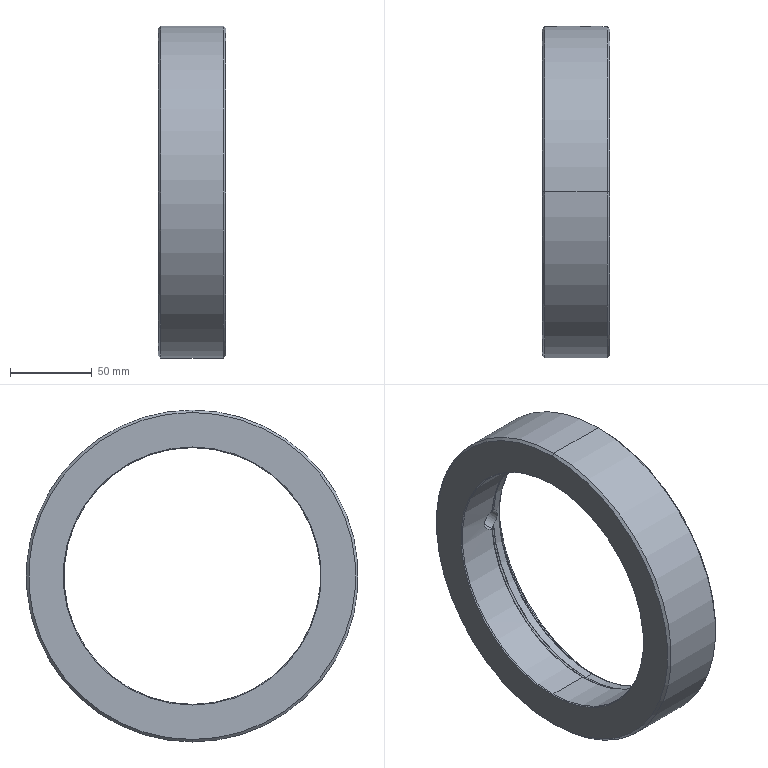Part | SolidWorks | features Chamfer 2, 3DProfileFeature 1, HoleWzd 1, Revolution 1 | 1 solid | 36 faces | box 41.402 x 203.2 x 203.2 mm | volume 502742 mm3 | torus 12 | cone 11 | cylinder 10 | plane 3 | commonest cylinder face diameters 12.573 x2 157.099 x2 160.274 x2 172.974 x2 203.2 x2
STEP:
#1=CARTESIAN_POINT('',(26.314,78.319,-6.287));
#2=VERTEX_POINT('',#1);
#3=CARTESIAN_POINT('',(26.136,78.298,-6.284));
#4=VERTEX_POINT('',#3);
#5=CARTESIAN_POINT('',(26.314,78.319,-6.287));
#6=CARTESIAN_POINT('',(26.256,78.305,-6.287));
#7=CARTESIAN_POINT('',(26.196,78.298,-6.286));
#8=CARTESIAN_POINT('',(26.136,78.298,-6.284));
#9=B_SPLINE_CURVE_WITH_KNOTS('',3,(#5,#6,#7,#8),.UNSPECIFIED.,.F.,.F.,(4,4),(0.0002182,0.0003967),.UNSPECIFIED.);
#10=EDGE_CURVE('',#2,#4,#9,.T.);
#11=ORIENTED_EDGE('',*,*,#10,.F.);
#12=CARTESIAN_POINT('',(26.314,101.405,-6.287));
#13=VERTEX_POINT('',#12);
#14=CARTESIAN_POINT('',(26.314,101.6,-6.287));
#15=DIRECTION('',(0.,1.,0.));
#16=VECTOR('',#15,1000.);
#17=LINE('',#14,#16);
#18=EDGE_CURVE('',#2,#13,#17,.T.);
#19=ORIENTED_EDGE('',*,*,#18,.T.);
#20=CARTESIAN_POINT('',(26.314,101.405,6.287));
#21=VERTEX_POINT('',#20);
#22=CARTESIAN_POINT('',(26.314,101.405,6.287));
#23=CARTESIAN_POINT('',(25.899,101.405,6.287));
#24=CARTESIAN_POINT('',(25.49,101.408,6.246));
#25=CARTESIAN_POINT('',(24.888,101.415,6.126));
#26=CARTESIAN_POINT('',(24.688,101.418,6.076));
#27=CARTESIAN_POINT('',(24.293,101.425,5.956));
#28=CARTESIAN_POINT('',(24.097,101.429,5.886));
#29=CARTESIAN_POINT('',(23.526,101.443,5.649));
#30=CARTESIAN_POINT('',(23.165,101.454,5.456));
#31=CARTESIAN_POINT('',(22.482,101.477,5.));
#32=CARTESIAN_POINT('',(22.158,101.49,4.734));
#33=CARTESIAN_POINT('',(21.578,101.515,4.154));
#34=CARTESIAN_POINT('',(21.318,101.528,3.838));
#35=CARTESIAN_POINT('',(20.974,101.546,3.323));
#36=CARTESIAN_POINT('',(20.867,101.552,3.144));
#37=CARTESIAN_POINT('',(20.673,101.562,2.781));
#38=CARTESIAN_POINT('',(20.497,101.572,2.41));
#39=CARTESIAN_POINT('',(20.359,101.58,2.025));
#40=CARTESIAN_POINT('',(20.24,101.587,1.631));
#41=CARTESIAN_POINT('',(20.189,101.59,1.429));
#42=CARTESIAN_POINT('',(20.068,101.597,0.8204));
#43=CARTESIAN_POINT('',(20.028,101.6,0.4124));
#44=CARTESIAN_POINT('',(20.028,101.6,-0.4079));
#45=CARTESIAN_POINT('',(20.069,101.597,-0.8245));
#46=CARTESIAN_POINT('',(20.229,101.588,-1.631));
#47=CARTESIAN_POINT('',(20.348,101.581,-2.023));
#48=CARTESIAN_POINT('',(20.584,101.567,-2.594));
#49=CARTESIAN_POINT('',(20.673,101.562,-2.782));
#50=CARTESIAN_POINT('',(20.868,101.551,-3.146));
#51=CARTESIAN_POINT('',(20.974,101.546,-3.322));
#52=CARTESIAN_POINT('',(21.315,101.528,-3.833));
#53=CARTESIAN_POINT('',(21.575,101.516,-4.151));
#54=CARTESIAN_POINT('',(22.162,101.49,-4.738));
#55=CARTESIAN_POINT('',(22.48,101.477,-4.998));
#56=CARTESIAN_POINT('',(22.99,101.46,-5.34));
#57=CARTESIAN_POINT('',(23.166,101.454,-5.445));
#58=CARTESIAN_POINT('',(23.53,101.443,-5.64));
#59=CARTESIAN_POINT('',(23.718,101.438,-5.729));
#60=CARTESIAN_POINT('',(24.29,101.425,-5.966));
#61=CARTESIAN_POINT('',(24.682,101.418,-6.085));
#62=CARTESIAN_POINT('',(25.487,101.408,-6.245));
#63=CARTESIAN_POINT('',(25.904,101.405,-6.287));
#64=CARTESIAN_POINT('',(26.314,101.405,-6.287));
#65=B_SPLINE_CURVE_WITH_KNOTS('',3,(#22,#23,#24,#25,#26,#27,#28,#29,#30,#31,#32,#33,#34,#35,#36,#37,#38,#39,#40,#41,#42,#43,#44,#45,#46,#47,#48,#49,#50,#51,#52,#53,#54,#55,#56,#57,#58,#59,#60,#61,#62,#63,#64),.UNSPECIFIED.,.F.,.F.,(4,2,2,2,2,2,2,2,1,2,2,2,2,2,2,2,2,2,2,2,2,4),(0.,0.001229,0.001843,0.002457,0.003686,0.004915,0.006144,0.006758,0.007372,0.007987,0.008601,0.00983,0.01106,0.01229,0.0129,0.01352,0.01474,0.01597,0.01659,0.0172,0.01843,0.01966),.UNSPECIFIED.);
#66=EDGE_CURVE('',#21,#13,#65,.T.);
#67=ORIENTED_EDGE('',*,*,#66,.F.);
#68=CARTESIAN_POINT('',(26.314,78.319,6.287));
#69=VERTEX_POINT('',#68);
#70=CARTESIAN_POINT('',(26.314,101.6,6.287));
#71=DIRECTION('',(0.,1.,0.));
#72=VECTOR('',#71,1000.);
#73=LINE('',#70,#72);
#74=EDGE_CURVE('',#69,#21,#73,.T.);
#75=ORIENTED_EDGE('',*,*,#74,.F.);
#76=CARTESIAN_POINT('',(26.136,78.298,6.284));
#77=VERTEX_POINT('',#76);
#78=CARTESIAN_POINT('',(26.136,78.298,6.284));
#79=CARTESIAN_POINT('',(26.196,78.298,6.286));
#80=CARTESIAN_POINT('',(26.256,78.305,6.287));
#81=CARTESIAN_POINT('',(26.314,78.319,6.287));
#82=B_SPLINE_CURVE_WITH_KNOTS('',3,(#78,#79,#80,#81),.UNSPECIFIED.,.F.,.F.,(4,4),(0.000000197,0.00018),.UNSPECIFIED.);
#83=EDGE_CURVE('',#77,#69,#82,.T.);
#84=ORIENTED_EDGE('',*,*,#83,.F.);
#85=CARTESIAN_POINT('',(26.136,78.298,-6.284));
#86=CARTESIAN_POINT('',(25.728,78.299,-6.272));
#87=CARTESIAN_POINT('',(25.328,78.303,-6.222));
#88=CARTESIAN_POINT('',(24.739,78.313,-6.089));
#89=CARTESIAN_POINT('',(24.545,78.317,-6.036));
#90=CARTESIAN_POINT('',(24.16,78.327,-5.909));
#91=CARTESIAN_POINT('',(23.969,78.332,-5.836));
#92=CARTESIAN_POINT('',(23.413,78.35,-5.592));
#93=CARTESIAN_POINT('',(23.062,78.364,-5.395));
#94=CARTESIAN_POINT('',(22.4,78.395,-4.936));
#95=CARTESIAN_POINT('',(22.086,78.411,-4.67));
#96=CARTESIAN_POINT('',(21.525,78.443,-4.092));
#97=CARTESIAN_POINT('',(21.274,78.459,-3.778));
#98=CARTESIAN_POINT('',(20.941,78.482,-3.27));
#99=CARTESIAN_POINT('',(20.838,78.489,-3.093));
#100=CARTESIAN_POINT('',(20.65,78.502,-2.735));
#101=CARTESIAN_POINT('',(20.565,78.508,-2.552));
#102=CARTESIAN_POINT('',(20.338,78.525,-1.993));
#103=CARTESIAN_POINT('',(20.223,78.534,-1.607));
#104=CARTESIAN_POINT('',(20.066,78.546,-0.8059));
#105=CARTESIAN_POINT('',(20.028,78.549,-0.4046));
#106=CARTESIAN_POINT('',(20.028,78.55,0.1989));
#107=CARTESIAN_POINT('',(20.037,78.549,0.4003));
#108=CARTESIAN_POINT('',(20.076,78.546,0.8036));
#109=CARTESIAN_POINT('',(20.106,78.543,1.006));
#110=CARTESIAN_POINT('',(20.222,78.534,1.603));
#111=CARTESIAN_POINT('',(20.337,78.525,1.988));
#112=CARTESIAN_POINT('',(20.64,78.503,2.735));
#113=CARTESIAN_POINT('',(20.83,78.489,3.099));
#114=CARTESIAN_POINT('',(21.271,78.46,3.774));
#115=CARTESIAN_POINT('',(21.522,78.444,4.088));
#116=CARTESIAN_POINT('',(21.945,78.419,4.524));
#117=CARTESIAN_POINT('',(22.094,78.411,4.664));
#118=CARTESIAN_POINT('',(22.403,78.395,4.926));
#119=CARTESIAN_POINT('',(22.563,78.387,5.048));
#120=CARTESIAN_POINT('',(23.058,78.365,5.392));
#121=CARTESIAN_POINT('',(23.41,78.351,5.59));
#122=CARTESIAN_POINT('',(24.156,78.326,5.918));
#123=CARTESIAN_POINT('',(24.539,78.317,6.044));
#124=CARTESIAN_POINT('',(25.323,78.303,6.221));
#125=CARTESIAN_POINT('',(25.728,78.299,6.272));
#126=CARTESIAN_POINT('',(26.136,78.298,6.284));
#127=B_SPLINE_CURVE_WITH_KNOTS('',3,(#85,#86,#87,#88,#89,#90,#91,#92,#93,#94,#95,#96,#97,#98,#99,#100,#101,#102,#103,#104,#105,#106,#107,#108,#109,#110,#111,#112,#113,#114,#115,#116,#117,#118,#119,#120,#121,#122,#123,#124,#125,#126),.UNSPECIFIED.,.F.,.F.,(4,2,2,2,2,2,2,2,2,2,2,2,2,2,2,2,2,2,2,2,4),(0.,0.001207,0.00181,0.002413,0.00362,0.004826,0.006033,0.006636,0.007239,0.008446,0.009653,0.01026,0.01086,0.01207,0.01327,0.01448,0.01508,0.01569,0.01689,0.0181,0.01931),.UNSPECIFIED.);
#128=EDGE_CURVE('',#4,#77,#127,.T.);
#129=ORIENTED_EDGE('',*,*,#128,.F.);
#130=EDGE_LOOP('',(#11,#19,#67,#75,#84,#129));
#131=FACE_OUTER_BOUND('',#130,.T.);
#132=CARTESIAN_POINT('',(26.314,101.6,0.));
#133=DIRECTION('',(0.,1.,0.));
#134=DIRECTION('',(0.,0.,1.));
#135=AXIS2_PLACEMENT_3D('',#132,#133,#134);
#136=CYLINDRICAL_SURFACE('',#135,6.287);
#137=ADVANCED_FACE('',(#131),#136,.F.);
#138=CARTESIAN_POINT('',(0.,0.,100.076));
#139=VERTEX_POINT('',#138);
#140=CARTESIAN_POINT('',(0.,0.,-100.076));
#141=VERTEX_POINT('',#140);
#142=CARTESIAN_POINT('',(0.,0.,0.));
#143=DIRECTION('',(-1.,0.,0.));
#144=DIRECTION('',(0.,0.,-1.));
#145=AXIS2_PLACEMENT_3D('',#142,#143,#144);
#146=CIRCLE('',#145,100.076);
#147=EDGE_CURVE('',#139,#141,#146,.T.);
#148=ORIENTED_EDGE('',*,*,#147,.F.);
#149=CARTESIAN_POINT('',(1.524,0.,101.6));
#150=VERTEX_POINT('',#149);
#151=CARTESIAN_POINT('',(0.,0.,100.076));
#152=DIRECTION('',(0.7071,0.,0.7071));
#153=VECTOR('',#152,1000.);
#154=LINE('',#151,#153);
#155=EDGE_CURVE('',#139,#150,#154,.T.);
#156=ORIENTED_EDGE('',*,*,#155,.T.);
#157=CARTESIAN_POINT('',(1.524,0.,-101.6));
#158=VERTEX_POINT('',#157);
#159=CARTESIAN_POINT('',(1.524,0.,0.));
#160=DIRECTION('',(1.,0.,0.));
#161=DIRECTION('',(0.,0.,-1.));
#162=AXIS2_PLACEMENT_3D('',#159,#160,#161);
#163=CIRCLE('',#162,101.6);
#164=EDGE_CURVE('',#158,#150,#163,.T.);
#165=ORIENTED_EDGE('',*,*,#164,.F.);
#166=CARTESIAN_POINT('',(0.,0.,-100.076));
#167=DIRECTION('',(0.7071,0.,-0.7071));
#168=VECTOR('',#167,1000.);
#169=LINE('',#166,#168);
#170=EDGE_CURVE('',#141,#158,#169,.T.);
#171=ORIENTED_EDGE('',*,*,#170,.F.);
#172=EDGE_LOOP('',(#148,#156,#165,#171));
#173=FACE_OUTER_BOUND('',#172,.T.);
#174=CARTESIAN_POINT('',(0.,0.,0.));
#175=DIRECTION('',(1.,0.,0.));
#176=DIRECTION('',(0.,0.,-1.));
#177=AXIS2_PLACEMENT_3D('',#174,#175,#176);
#178=CONICAL_SURFACE('',#177,100.076,0.7854);
#179=ADVANCED_FACE('',(#173),#178,.T.);
#180=CARTESIAN_POINT('',(41.402,0.,-100.076));
#181=VERTEX_POINT('',#180);
#182=CARTESIAN_POINT('',(41.402,0.,100.076));
#183=VERTEX_POINT('',#182);
#184=CARTESIAN_POINT('',(41.402,0.,0.));
#185=DIRECTION('',(1.,0.,0.));
#186=DIRECTION('',(0.,0.,1.));
#187=AXIS2_PLACEMENT_3D('',#184,#185,#186);
#188=CIRCLE('',#187,100.076);
#189=EDGE_CURVE('',#181,#183,#188,.T.);
#190=ORIENTED_EDGE('',*,*,#189,.F.);
#191=CARTESIAN_POINT('',(39.878,0.,-101.6));
#192=VERTEX_POINT('',#191);
#193=CARTESIAN_POINT('',(39.878,0.,-101.6));
#194=DIRECTION('',(-0.7071,0.,-0.7071));
#195=VECTOR('',#194,1000.);
#196=LINE('',#193,#195);
#197=EDGE_CURVE('',#181,#192,#196,.T.);
#198=ORIENTED_EDGE('',*,*,#197,.T.);
#199=CARTESIAN_POINT('',(39.878,0.,101.6));
#200=VERTEX_POINT('',#199);
#201=CARTESIAN_POINT('',(39.878,0.,0.));
#202=DIRECTION('',(-1.,0.,0.));
#203=DIRECTION('',(0.,0.,1.));
#204=AXIS2_PLACEMENT_3D('',#201,#202,#203);
#205=CIRCLE('',#204,101.6);
#206=EDGE_CURVE('',#200,#192,#205,.T.);
#207=ORIENTED_EDGE('',*,*,#206,.F.);
#208=CARTESIAN_POINT('',(39.878,0.,101.6));
#209=DIRECTION('',(-0.7071,0.,0.7071));
#210=VECTOR('',#209,1000.);
#211=LINE('',#208,#210);
#212=EDGE_CURVE('',#183,#200,#211,.T.);
#213=ORIENTED_EDGE('',*,*,#212,.F.);
#214=EDGE_LOOP('',(#190,#198,#207,#213));
#215=FACE_OUTER_BOUND('',#214,.T.);
#216=CARTESIAN_POINT('',(39.878,0.,0.));
#217=DIRECTION('',(-1.,0.,0.));
#218=DIRECTION('',(0.,0.,1.));
#219=AXIS2_PLACEMENT_3D('',#216,#217,#218);
#220=CONICAL_SURFACE('',#219,101.6,0.7854);
#221=ADVANCED_FACE('',(#215),#220,.T.);
#222=CARTESIAN_POINT('',(0.762,0.,-78.549));
#223=VERTEX_POINT('',#222);
#224=CARTESIAN_POINT('',(0.762,0.,78.549));
#225=VERTEX_POINT('',#224);
#226=CARTESIAN_POINT('',(0.762,0.,0.));
#227=DIRECTION('',(-1.,0.,0.));
#228=DIRECTION('',(0.,0.,-1.));
#229=AXIS2_PLACEMENT_3D('',#226,#227,#228);
#230=CIRCLE('',#229,78.549);
#231=EDGE_CURVE('',#223,#225,#230,.T.);
#232=ORIENTED_EDGE('',*,*,#231,.F.);
#233=CARTESIAN_POINT('',(0.,0.,-78.989));
#234=VERTEX_POINT('',#233);
#235=CARTESIAN_POINT('',(0.762,0.,-78.549));
#236=DIRECTION('',(-0.866,0.,-0.5));
#237=VECTOR('',#236,1000.);
#238=LINE('',#235,#237);
#239=EDGE_CURVE('',#223,#234,#238,.T.);
#240=ORIENTED_EDGE('',*,*,#239,.T.);
#241=CARTESIAN_POINT('',(0.,0.,78.989));
#242=VERTEX_POINT('',#241);
#243=CARTESIAN_POINT('',(0.,0.,0.));
#244=DIRECTION('',(1.,0.,0.));
#245=DIRECTION('',(0.,0.,-1.));
#246=AXIS2_PLACEMENT_3D('',#243,#244,#245);
#247=CIRCLE('',#246,78.989);
#248=EDGE_CURVE('',#242,#234,#247,.T.);
#249=ORIENTED_EDGE('',*,*,#248,.F.);
#250=CARTESIAN_POINT('',(0.762,0.,78.549));
#251=DIRECTION('',(-0.866,0.,0.5));
#252=VECTOR('',#251,1000.);
#253=LINE('',#250,#252);
#254=EDGE_CURVE('',#225,#242,#253,.T.);
#255=ORIENTED_EDGE('',*,*,#254,.F.);
#256=EDGE_LOOP('',(#232,#240,#249,#255));
#257=FACE_OUTER_BOUND('',#256,.T.);
#258=CARTESIAN_POINT('',(0.762,0.,0.));
#259=DIRECTION('',(-1.,0.,0.));
#260=DIRECTION('',(0.,0.,1.));
#261=AXIS2_PLACEMENT_3D('',#258,#259,#260);
#262=CONICAL_SURFACE('',#261,78.549,0.5236);
#263=ADVANCED_FACE('',(#257),#262,.F.);
#264=CARTESIAN_POINT('',(26.136,0.,-78.549));
#265=VERTEX_POINT('',#264);
#266=CARTESIAN_POINT('',(26.136,0.,78.549));
#267=VERTEX_POINT('',#266);
#268=CARTESIAN_POINT('',(26.136,0.,0.));
#269=DIRECTION('',(-1.,0.,0.));
#270=DIRECTION('',(0.,0.,1.));
#271=AXIS2_PLACEMENT_3D('',#268,#269,#270);
#272=CIRCLE('',#271,78.549);
#273=EDGE_CURVE('',#265,#267,#272,.T.);
#274=ORIENTED_EDGE('',*,*,#273,.F.);
#275=CARTESIAN_POINT('',(-48.08,0.,-78.549));
#276=DIRECTION('',(-1.,0.,0.));
#277=VECTOR('',#276,1000.);
#278=LINE('',#275,#277);
#279=EDGE_CURVE('',#265,#223,#278,.T.);
#280=ORIENTED_EDGE('',*,*,#279,.T.);
#281=ORIENTED_EDGE('',*,*,#231,.T.);
#282=CARTESIAN_POINT('',(-48.08,0.,78.549));
#283=DIRECTION('',(-1.,0.,0.));
#284=VECTOR('',#283,1000.);
#285=LINE('',#282,#284);
#286=EDGE_CURVE('',#267,#225,#285,.T.);
#287=ORIENTED_EDGE('',*,*,#286,.F.);
#288=EDGE_LOOP('',(#274,#280,#281,#287));
#289=FACE_OUTER_BOUND('',#288,.T.);
#290=CARTESIAN_POINT('',(-48.08,0.,0.));
#291=DIRECTION('',(-1.,0.,0.));
#292=DIRECTION('',(0.,0.,1.));
#293=AXIS2_PLACEMENT_3D('',#290,#291,#292);
#294=CYLINDRICAL_SURFACE('',#293,78.549);
#295=ADVANCED_FACE('',(#289),#294,.F.);
#296=CARTESIAN_POINT('',(26.136,0.,0.));
#297=DIRECTION('',(-1.,0.,0.));
#298=DIRECTION('',(0.,0.,1.));
#299=AXIS2_PLACEMENT_3D('',#296,#297,#298);
#300=CIRCLE('',#299,78.549);
#301=EDGE_CURVE('',#4,#265,#300,.T.);
#302=ORIENTED_EDGE('',*,*,#301,.T.);
#303=CARTESIAN_POINT('',(26.517,0.,-78.652));
#304=VERTEX_POINT('',#303);
#305=CARTESIAN_POINT('',(26.136,0.,-79.311));
#306=DIRECTION('',(0.,1.,0.));
#307=DIRECTION('',(0.,0.,1.));
#308=AXIS2_PLACEMENT_3D('',#305,#306,#307);
#309=CIRCLE('',#308,0.762);
#310=EDGE_CURVE('',#265,#304,#309,.T.);
#311=ORIENTED_EDGE('',*,*,#310,.T.);
#312=CARTESIAN_POINT('',(26.517,78.4,-6.283));
#313=VERTEX_POINT('',#312);
#314=CARTESIAN_POINT('',(26.517,0.,0.));
#315=DIRECTION('',(-1.,0.,0.));
#316=DIRECTION('',(0.,0.,1.));
#317=AXIS2_PLACEMENT_3D('',#314,#315,#316);
#318=CIRCLE('',#317,78.652);
#319=EDGE_CURVE('',#313,#304,#318,.T.);
#320=ORIENTED_EDGE('',*,*,#319,.F.);
#321=CARTESIAN_POINT('',(26.517,78.4,-6.283));
#322=CARTESIAN_POINT('',(26.453,78.363,-6.285));
#323=CARTESIAN_POINT('',(26.386,78.336,-6.287));
#324=CARTESIAN_POINT('',(26.314,78.319,-6.287));
#325=B_SPLINE_CURVE_WITH_KNOTS('',3,(#321,#322,#323,#324),.UNSPECIFIED.,.F.,.F.,(4,4),(0.000000228,0.0002182),.UNSPECIFIED.);
#326=EDGE_CURVE('',#313,#2,#325,.T.);
#327=ORIENTED_EDGE('',*,*,#326,.T.);
#328=ORIENTED_EDGE('',*,*,#10,.T.);
#329=EDGE_LOOP('',(#302,#311,#320,#327,#328));
#330=FACE_OUTER_BOUND('',#329,.T.);
#331=CARTESIAN_POINT('',(26.136,0.,0.));
#332=DIRECTION('',(-1.,0.,0.));
#333=DIRECTION('',(0.,0.,1.));
#334=AXIS2_PLACEMENT_3D('',#331,#332,#333);
#335=TOROIDAL_SURFACE('',#334,79.311,0.762);
#336=ADVANCED_FACE('',(#330),#335,.T.);
#337=ORIENTED_EDGE('',*,*,#310,.F.);
#338=ORIENTED_EDGE('',*,*,#273,.T.);
#339=CARTESIAN_POINT('',(26.517,0.,78.652));
#340=VERTEX_POINT('',#339);
#341=CARTESIAN_POINT('',(26.136,0.,79.311));
#342=DIRECTION('',(0.,-1.,0.));
#343=DIRECTION('',(0.,0.,-1.));
#344=AXIS2_PLACEMENT_3D('',#341,#342,#343);
#345=CIRCLE('',#344,0.762);
#346=EDGE_CURVE('',#267,#340,#345,.T.);
#347=ORIENTED_EDGE('',*,*,#346,.T.);
#348=CARTESIAN_POINT('',(26.517,0.,0.));
#349=DIRECTION('',(-1.,0.,0.));
#350=DIRECTION('',(0.,0.,1.));
#351=AXIS2_PLACEMENT_3D('',#348,#349,#350);
#352=CIRCLE('',#351,78.652);
#353=EDGE_CURVE('',#304,#340,#352,.T.);
#354=ORIENTED_EDGE('',*,*,#353,.F.);
#355=EDGE_LOOP('',(#337,#338,#347,#354));
#356=FACE_OUTER_BOUND('',#355,.T.);
#357=CARTESIAN_POINT('',(26.136,0.,0.));
#358=DIRECTION('',(-1.,0.,0.));
#359=DIRECTION('',(0.,0.,1.));
#360=AXIS2_PLACEMENT_3D('',#357,#358,#359);
#361=TOROIDAL_SURFACE('',#360,79.311,0.762);
#362=ADVANCED_FACE('',(#356),#361,.T.);
#363=ORIENTED_EDGE('',*,*,#353,.T.);
#364=CARTESIAN_POINT('',(28.913,0.,80.035));
#365=VERTEX_POINT('',#364);
#366=CARTESIAN_POINT('',(26.517,0.,78.652));
#367=DIRECTION('',(0.866,0.,0.5));
#368=VECTOR('',#367,1000.);
#369=LINE('',#366,#368);
#370=EDGE_CURVE('',#340,#365,#369,.T.);
#371=ORIENTED_EDGE('',*,*,#370,.T.);
#372=CARTESIAN_POINT('',(28.913,0.,-80.035));
#373=VERTEX_POINT('',#372);
#374=CARTESIAN_POINT('',(28.913,0.,0.));
#375=DIRECTION('',(-1.,0.,0.));
#376=DIRECTION('',(0.,0.,1.));
#377=AXIS2_PLACEMENT_3D('',#374,#375,#376);
#378=CIRCLE('',#377,80.035);
#379=EDGE_CURVE('',#373,#365,#378,.T.);
#380=ORIENTED_EDGE('',*,*,#379,.F.);
#381=CARTESIAN_POINT('',(26.517,0.,-78.652));
#382=DIRECTION('',(0.866,0.,-0.5));
#383=VECTOR('',#382,1000.);
#384=LINE('',#381,#383);
#385=EDGE_CURVE('',#304,#373,#384,.T.);
#386=ORIENTED_EDGE('',*,*,#385,.F.);
#387=EDGE_LOOP('',(#363,#371,#380,#386));
#388=FACE_OUTER_BOUND('',#387,.T.);
#389=CARTESIAN_POINT('',(26.517,0.,0.));
#390=DIRECTION('',(1.,0.,0.));
#391=DIRECTION('',(0.,0.,-1.));
#392=AXIS2_PLACEMENT_3D('',#389,#390,#391);
#393=CONICAL_SURFACE('',#392,78.652,0.5236);
#394=ADVANCED_FACE('',(#388),#393,.F.);
#395=ORIENTED_EDGE('',*,*,#319,.T.);
#396=ORIENTED_EDGE('',*,*,#385,.T.);
#397=CARTESIAN_POINT('',(28.913,79.83,-5.725));
#398=VERTEX_POINT('',#397);
#399=CARTESIAN_POINT('',(28.913,0.,0.));
#400=DIRECTION('',(-1.,0.,0.));
#401=DIRECTION('',(0.,0.,1.));
#402=AXIS2_PLACEMENT_3D('',#399,#400,#401);
#403=CIRCLE('',#402,80.035);
#404=EDGE_CURVE('',#398,#373,#403,.T.);
#405=ORIENTED_EDGE('',*,*,#404,.F.);
#406=CARTESIAN_POINT('',(28.913,79.83,-5.725));
#407=CARTESIAN_POINT('',(28.532,79.597,-5.897));
#408=CARTESIAN_POINT('',(28.142,79.361,-6.029));
#409=CARTESIAN_POINT('',(27.343,78.884,-6.215));
#410=CARTESIAN_POINT('',(26.932,78.642,-6.27));
#411=CARTESIAN_POINT('',(26.517,78.4,-6.283));
#412=B_SPLINE_CURVE_WITH_KNOTS('',3,(#406,#407,#408,#409,#410,#411),.UNSPECIFIED.,.F.,.F.,(4,2,4),(0.0003004,0.001723,0.003145),.UNSPECIFIED.);
#413=EDGE_CURVE('',#398,#313,#412,.T.);
#414=ORIENTED_EDGE('',*,*,#413,.T.);
#415=EDGE_LOOP('',(#395,#396,#405,#414));
#416=FACE_OUTER_BOUND('',#415,.T.);
#417=CARTESIAN_POINT('',(26.517,0.,0.));
#418=DIRECTION('',(1.,0.,0.));
#419=DIRECTION('',(0.,0.,-1.));
#420=AXIS2_PLACEMENT_3D('',#417,#418,#419);
#421=CONICAL_SURFACE('',#420,78.652,0.5236);
#422=ADVANCED_FACE('',(#416),#421,.F.);
#423=CARTESIAN_POINT('',(29.294,0.,-80.137));
#424=VERTEX_POINT('',#423);
#425=CARTESIAN_POINT('',(29.294,0.,80.137));
#426=VERTEX_POINT('',#425);
#427=CARTESIAN_POINT('',(29.294,0.,0.));
#428=DIRECTION('',(-1.,0.,0.));
#429=DIRECTION('',(0.,0.,1.));
#430=AXIS2_PLACEMENT_3D('',#427,#428,#429);
#431=CIRCLE('',#430,80.137);
#432=EDGE_CURVE('',#424,#426,#431,.T.);
#433=ORIENTED_EDGE('',*,*,#432,.F.);
#434=CARTESIAN_POINT('',(29.294,0.,-79.375));
#435=DIRECTION('',(0.,1.,0.));
#436=DIRECTION('',(0.,0.,1.));
#437=AXIS2_PLACEMENT_3D('',#434,#435,#436);
#438=CIRCLE('',#437,0.762);
#439=EDGE_CURVE('',#424,#373,#438,.T.);
#440=ORIENTED_EDGE('',*,*,#439,.T.);
#441=ORIENTED_EDGE('',*,*,#379,.T.);
#442=CARTESIAN_POINT('',(29.294,0.,79.375));
#443=DIRECTION('',(0.,-1.,0.));
#444=DIRECTION('',(0.,0.,-1.));
#445=AXIS2_PLACEMENT_3D('',#442,#443,#444);
#446=CIRCLE('',#445,0.762);
#447=EDGE_CURVE('',#426,#365,#446,.T.);
#448=ORIENTED_EDGE('',*,*,#447,.F.);
#449=EDGE_LOOP('',(#433,#440,#441,#448));
#450=FACE_OUTER_BOUND('',#449,.T.);
#451=CARTESIAN_POINT('',(29.294,0.,0.));
#452=DIRECTION('',(-1.,0.,0.));
#453=DIRECTION('',(0.,0.,1.));
#454=AXIS2_PLACEMENT_3D('',#451,#452,#453);
#455=TOROIDAL_SURFACE('',#454,79.375,0.762);
#456=ADVANCED_FACE('',(#450),#455,.F.);
#457=CARTESIAN_POINT('',(29.294,79.946,5.536));
#458=VERTEX_POINT('',#457);
#459=CARTESIAN_POINT('',(29.294,0.,0.));
#460=DIRECTION('',(-1.,0.,0.));
#461=DIRECTION('',(0.,0.,1.));
#462=AXIS2_PLACEMENT_3D('',#459,#460,#461);
#463=CIRCLE('',#462,80.137);
#464=EDGE_CURVE('',#426,#458,#463,.T.);
#465=ORIENTED_EDGE('',*,*,#464,.F.);
#466=ORIENTED_EDGE('',*,*,#447,.T.);
#467=CARTESIAN_POINT('',(28.913,79.83,5.725));
#468=VERTEX_POINT('',#467);
#469=CARTESIAN_POINT('',(28.913,0.,0.));
#470=DIRECTION('',(-1.,0.,0.));
#471=DIRECTION('',(0.,0.,1.));
#472=AXIS2_PLACEMENT_3D('',#469,#470,#471);
#473=CIRCLE('',#472,80.035);
#474=EDGE_CURVE('',#365,#468,#473,.T.);
#475=ORIENTED_EDGE('',*,*,#474,.T.);
#476=CARTESIAN_POINT('',(28.913,79.83,5.725));
#477=CARTESIAN_POINT('',(29.032,79.903,5.671));
#478=CARTESIAN_POINT('',(29.162,79.941,5.607));
#479=CARTESIAN_POINT('',(29.294,79.946,5.536));
#480=B_SPLINE_CURVE_WITH_KNOTS('',3,(#476,#477,#478,#479),.UNSPECIFIED.,.F.,.F.,(4,4),(0.000000248,0.0004419),.UNSPECIFIED.);
#481=EDGE_CURVE('',#468,#458,#480,.T.);
#482=ORIENTED_EDGE('',*,*,#481,.T.);
#483=EDGE_LOOP('',(#465,#466,#475,#482));
#484=FACE_OUTER_BOUND('',#483,.T.);
#485=CARTESIAN_POINT('',(29.294,0.,0.));
#486=DIRECTION('',(-1.,0.,0.));
#487=DIRECTION('',(0.,0.,1.));
#488=AXIS2_PLACEMENT_3D('',#485,#486,#487);
#489=TOROIDAL_SURFACE('',#488,79.375,0.762);
#490=ADVANCED_FACE('',(#484),#489,.F.);
#491=CARTESIAN_POINT('',(34.163,0.,-80.137));
#492=VERTEX_POINT('',#491);
#493=CARTESIAN_POINT('',(34.163,0.,80.137));
#494=VERTEX_POINT('',#493);
#495=CARTESIAN_POINT('',(34.163,0.,0.));
#496=DIRECTION('',(-1.,0.,0.));
#497=DIRECTION('',(0.,0.,1.));
#498=AXIS2_PLACEMENT_3D('',#495,#496,#497);
#499=CIRCLE('',#498,80.137);
#500=EDGE_CURVE('',#492,#494,#499,.T.);
#501=ORIENTED_EDGE('',*,*,#500,.F.);
#502=CARTESIAN_POINT('',(-48.08,0.,-80.137));
#503=DIRECTION('',(-1.,0.,0.));
#504=VECTOR('',#503,1000.);
#505=LINE('',#502,#504);
#506=EDGE_CURVE('',#492,#424,#505,.T.);
#507=ORIENTED_EDGE('',*,*,#506,.T.);
#508=ORIENTED_EDGE('',*,*,#432,.T.);
#509=CARTESIAN_POINT('',(-48.08,0.,80.137));
#510=DIRECTION('',(-1.,0.,0.));
#511=VECTOR('',#510,1000.);
#512=LINE('',#509,#511);
#513=EDGE_CURVE('',#494,#426,#512,.T.);
#514=ORIENTED_EDGE('',*,*,#513,.F.);
#515=EDGE_LOOP('',(#501,#507,#508,#514));
#516=FACE_OUTER_BOUND('',#515,.T.);
#517=CARTESIAN_POINT('',(-48.08,0.,0.));
#518=DIRECTION('',(-1.,0.,0.));
#519=DIRECTION('',(0.,0.,1.));
#520=AXIS2_PLACEMENT_3D('',#517,#518,#519);
#521=CYLINDRICAL_SURFACE('',#520,80.137);
#522=ADVANCED_FACE('',(#516),#521,.F.);
#523=CARTESIAN_POINT('',(34.163,0.,0.));
#524=DIRECTION('',(-1.,0.,0.));
#525=DIRECTION('',(0.,0.,1.));
#526=AXIS2_PLACEMENT_3D('',#523,#524,#525);
#527=CIRCLE('',#526,80.137);
#528=EDGE_CURVE('',#494,#492,#527,.T.);
#529=ORIENTED_EDGE('',*,*,#528,.T.);
#530=CARTESIAN_POINT('',(34.925,0.,-80.899));
#531=VERTEX_POINT('',#530);
#532=CARTESIAN_POINT('',(34.163,0.,-80.899));
#533=DIRECTION('',(0.,1.,0.));
#534=DIRECTION('',(0.,0.,1.));
#535=AXIS2_PLACEMENT_3D('',#532,#533,#534);
#536=CIRCLE('',#535,0.762);
#537=EDGE_CURVE('',#492,#531,#536,.T.);
#538=ORIENTED_EDGE('',*,*,#537,.T.);
#539=CARTESIAN_POINT('',(34.925,0.,80.899));
#540=VERTEX_POINT('',#539);
#541=CARTESIAN_POINT('',(34.925,0.,0.));
#542=DIRECTION('',(-1.,0.,0.));
#543=DIRECTION('',(0.,0.,1.));
#544=AXIS2_PLACEMENT_3D('',#541,#542,#543);
#545=CIRCLE('',#544,80.899);
#546=EDGE_CURVE('',#540,#531,#545,.T.);
#547=ORIENTED_EDGE('',*,*,#546,.F.);
#548=CARTESIAN_POINT('',(34.163,0.,80.899));
#549=DIRECTION('',(0.,-1.,0.));
#550=DIRECTION('',(0.,0.,-1.));
#551=AXIS2_PLACEMENT_3D('',#548,#549,#550);
#552=CIRCLE('',#551,0.762);
#553=EDGE_CURVE('',#494,#540,#552,.T.);
#554=ORIENTED_EDGE('',*,*,#553,.F.);
#555=EDGE_LOOP('',(#529,#538,#547,#554));
#556=FACE_OUTER_BOUND('',#555,.T.);
#557=CARTESIAN_POINT('',(34.163,0.,0.));
#558=DIRECTION('',(-1.,0.,0.));
#559=DIRECTION('',(0.,0.,1.));
#560=AXIS2_PLACEMENT_3D('',#557,#558,#559);
#561=TOROIDAL_SURFACE('',#560,80.899,0.762);
#562=ADVANCED_FACE('',(#556),#561,.T.);
#563=CARTESIAN_POINT('',(35.884,0.,-86.893));
#564=VERTEX_POINT('',#563);
#565=CARTESIAN_POINT('',(35.884,0.,86.893));
#566=VERTEX_POINT('',#565);
#567=CARTESIAN_POINT('',(35.884,0.,0.));
#568=DIRECTION('',(-1.,0.,0.));
#569=DIRECTION('',(0.,0.,1.));
#570=AXIS2_PLACEMENT_3D('',#567,#568,#569);
#571=CIRCLE('',#570,86.893);
#572=EDGE_CURVE('',#564,#566,#571,.T.);
#573=ORIENTED_EDGE('',*,*,#572,.F.);
#574=CARTESIAN_POINT('',(34.925,0.,-86.157));
#575=VERTEX_POINT('',#574);
#576=CARTESIAN_POINT('',(35.687,0.,-86.157));
#577=DIRECTION('',(0.,1.,0.));
#578=DIRECTION('',(0.,0.,1.));
#579=AXIS2_PLACEMENT_3D('',#576,#577,#578);
#580=CIRCLE('',#579,0.762);
#581=EDGE_CURVE('',#564,#575,#580,.T.);
#582=ORIENTED_EDGE('',*,*,#581,.T.);
#583=CARTESIAN_POINT('',(34.925,0.,86.157));
#584=VERTEX_POINT('',#583);
#585=CARTESIAN_POINT('',(34.925,0.,0.));
#586=DIRECTION('',(-1.,0.,0.));
#587=DIRECTION('',(0.,0.,1.));
#588=AXIS2_PLACEMENT_3D('',#585,#586,#587);
#589=CIRCLE('',#588,86.157);
#590=EDGE_CURVE('',#575,#584,#589,.T.);
#591=ORIENTED_EDGE('',*,*,#590,.T.);
#592=CARTESIAN_POINT('',(35.687,0.,86.157));
#593=DIRECTION('',(0.,-1.,0.));
#594=DIRECTION('',(0.,0.,-1.));
#595=AXIS2_PLACEMENT_3D('',#592,#593,#594);
#596=CIRCLE('',#595,0.762);
#597=EDGE_CURVE('',#566,#584,#596,.T.);
#598=ORIENTED_EDGE('',*,*,#597,.F.);
#599=EDGE_LOOP('',(#573,#582,#591,#598));
#600=FACE_OUTER_BOUND('',#599,.T.);
#601=CARTESIAN_POINT('',(35.687,0.,0.));
#602=DIRECTION('',(-1.,0.,0.));
#603=DIRECTION('',(0.,0.,1.));
#604=AXIS2_PLACEMENT_3D('',#601,#602,#603);
#605=TOROIDAL_SURFACE('',#604,86.157,0.762);
#606=ADVANCED_FACE('',(#600),#605,.F.);
#607=CARTESIAN_POINT('',(37.401,0.,-86.487));
#608=VERTEX_POINT('',#607);
#609=CARTESIAN_POINT('',(37.401,0.,86.487));
#610=VERTEX_POINT('',#609);
#611=CARTESIAN_POINT('',(37.401,0.,0.));
#612=DIRECTION('',(-1.,0.,0.));
#613=DIRECTION('',(0.,0.,1.));
#614=AXIS2_PLACEMENT_3D('',#611,#612,#613);
#615=CIRCLE('',#614,86.487);
#616=EDGE_CURVE('',#608,#610,#615,.T.);
#617=ORIENTED_EDGE('',*,*,#616,.F.);
#618=CARTESIAN_POINT('',(35.884,0.,-86.893));
#619=DIRECTION('',(-0.9659,0.,-0.2588));
#620=VECTOR('',#619,1000.);
#621=LINE('',#618,#620);
#622=EDGE_CURVE('',#608,#564,#621,.T.);
#623=ORIENTED_EDGE('',*,*,#622,.T.);
#624=ORIENTED_EDGE('',*,*,#572,.T.);
#625=CARTESIAN_POINT('',(35.884,0.,86.893));
#626=DIRECTION('',(-0.9659,0.,0.2588));
#627=VECTOR('',#626,1000.);
#628=LINE('',#625,#627);
#629=EDGE_CURVE('',#610,#566,#628,.T.);
#630=ORIENTED_EDGE('',*,*,#629,.F.);
#631=EDGE_LOOP('',(#617,#623,#624,#630));
#632=FACE_OUTER_BOUND('',#631,.T.);
#633=CARTESIAN_POINT('',(35.884,0.,0.));
#634=DIRECTION('',(-1.,0.,0.));
#635=DIRECTION('',(0.,0.,1.));
#636=AXIS2_PLACEMENT_3D('',#633,#634,#635);
#637=CONICAL_SURFACE('',#636,86.893,0.2618);
#638=ADVANCED_FACE('',(#632),#637,.F.);
#639=CARTESIAN_POINT('',(39.878,0.,-86.487));
#640=VERTEX_POINT('',#639);
#641=CARTESIAN_POINT('',(39.878,0.,86.487));
#642=VERTEX_POINT('',#641);
#643=CARTESIAN_POINT('',(39.878,0.,0.));
#644=DIRECTION('',(-1.,0.,0.));
#645=DIRECTION('',(0.,0.,1.));
#646=AXIS2_PLACEMENT_3D('',#643,#644,#645);
#647=CIRCLE('',#646,86.487);
#648=EDGE_CURVE('',#640,#642,#647,.T.);
#649=ORIENTED_EDGE('',*,*,#648,.F.);
#650=CARTESIAN_POINT('',(-48.08,0.,-86.487));
#651=DIRECTION('',(-1.,0.,0.));
#652=VECTOR('',#651,1000.);
#653=LINE('',#650,#652);
#654=EDGE_CURVE('',#640,#608,#653,.T.);
#655=ORIENTED_EDGE('',*,*,#654,.T.);
#656=ORIENTED_EDGE('',*,*,#616,.T.);
#657=CARTESIAN_POINT('',(-48.08,0.,86.487));
#658=DIRECTION('',(-1.,0.,0.));
#659=VECTOR('',#658,1000.);
#660=LINE('',#657,#659);
#661=EDGE_CURVE('',#642,#610,#660,.T.);
#662=ORIENTED_EDGE('',*,*,#661,.F.);
#663=EDGE_LOOP('',(#649,#655,#656,#662));
#664=FACE_OUTER_BOUND('',#663,.T.);
#665=CARTESIAN_POINT('',(-48.08,0.,0.));
#666=DIRECTION('',(-1.,0.,0.));
#667=DIRECTION('',(0.,0.,1.));
#668=AXIS2_PLACEMENT_3D('',#665,#666,#667);
#669=CYLINDRICAL_SURFACE('',#668,86.487);
#670=ADVANCED_FACE('',(#664),#669,.F.);
#671=CARTESIAN_POINT('',(39.878,0.,0.));
#672=DIRECTION('',(-1.,0.,0.));
#673=DIRECTION('',(0.,0.,1.));
#674=AXIS2_PLACEMENT_3D('',#671,#672,#673);
#675=CIRCLE('',#674,86.487);
#676=EDGE_CURVE('',#642,#640,#675,.T.);
#677=ORIENTED_EDGE('',*,*,#676,.T.);
#678=CARTESIAN_POINT('',(41.402,0.,-88.011));
#679=VERTEX_POINT('',#678);
#680=CARTESIAN_POINT('',(39.878,0.,-88.011));
#681=DIRECTION('',(0.,1.,0.));
#682=DIRECTION('',(0.,0.,1.));
#683=AXIS2_PLACEMENT_3D('',#680,#681,#682);
#684=CIRCLE('',#683,1.524);
#685=EDGE_CURVE('',#640,#679,#684,.T.);
#686=ORIENTED_EDGE('',*,*,#685,.T.);
#687=CARTESIAN_POINT('',(41.402,0.,88.011));
#688=VERTEX_POINT('',#687);
#689=CARTESIAN_POINT('',(41.402,0.,0.));
#690=DIRECTION('',(-1.,0.,0.));
#691=DIRECTION('',(0.,0.,1.));
#692=AXIS2_PLACEMENT_3D('',#689,#690,#691);
#693=CIRCLE('',#692,88.011);
#694=EDGE_CURVE('',#688,#679,#693,.T.);
#695=ORIENTED_EDGE('',*,*,#694,.F.);
#696=CARTESIAN_POINT('',(39.878,0.,88.011));
#697=DIRECTION('',(0.,-1.,0.));
#698=DIRECTION('',(0.,0.,-1.));
#699=AXIS2_PLACEMENT_3D('',#696,#697,#698);
#700=CIRCLE('',#699,1.524);
#701=EDGE_CURVE('',#642,#688,#700,.T.);
#702=ORIENTED_EDGE('',*,*,#701,.F.);
#703=EDGE_LOOP('',(#677,#686,#695,#702));
#704=FACE_OUTER_BOUND('',#703,.T.);
#705=CARTESIAN_POINT('',(39.878,0.,0.));
#706=DIRECTION('',(-1.,0.,0.));
#707=DIRECTION('',(0.,0.,1.));
#708=AXIS2_PLACEMENT_3D('',#705,#706,#707);
#709=TOROIDAL_SURFACE('',#708,88.011,1.524);
#710=ADVANCED_FACE('',(#704),#709,.T.);
#711=ORIENTED_EDGE('',*,*,#66,.T.);
#712=CARTESIAN_POINT('',(26.314,101.405,-6.287));
#713=CARTESIAN_POINT('',(26.725,101.405,-6.287));
#714=CARTESIAN_POINT('',(27.132,101.408,-6.247));
#715=CARTESIAN_POINT('',(27.74,101.415,-6.126));
#716=CARTESIAN_POINT('',(27.942,101.418,-6.076));
#717=CARTESIAN_POINT('',(28.336,101.425,-5.956));
#718=CARTESIAN_POINT('',(28.529,101.429,-5.887));
#719=CARTESIAN_POINT('',(29.097,101.443,-5.652));
#720=CARTESIAN_POINT('',(29.462,101.454,-5.458));
#721=CARTESIAN_POINT('',(30.15,101.477,-4.998));
#722=CARTESIAN_POINT('',(30.467,101.49,-4.738));
#723=CARTESIAN_POINT('',(31.047,101.515,-4.159));
#724=CARTESIAN_POINT('',(31.312,101.528,-3.836));
#725=CARTESIAN_POINT('',(31.769,101.552,-3.152));
#726=CARTESIAN_POINT('',(31.962,101.562,-2.792));
#727=CARTESIAN_POINT('',(32.199,101.576,-2.221));
#728=CARTESIAN_POINT('',(32.269,101.58,-2.025));
#729=CARTESIAN_POINT('',(32.389,101.587,-1.63));
#730=CARTESIAN_POINT('',(32.439,101.59,-1.431));
#731=CARTESIAN_POINT('',(32.56,101.597,-0.8281));
#732=CARTESIAN_POINT('',(32.601,101.6,-0.4199));
#733=CARTESIAN_POINT('',(32.601,101.6,0.4097));
#734=CARTESIAN_POINT('',(32.561,101.597,0.8195));
#735=CARTESIAN_POINT('',(32.441,101.59,1.422));
#736=CARTESIAN_POINT('',(32.392,101.587,1.621));
#737=CARTESIAN_POINT('',(32.273,101.58,2.016));
#738=CARTESIAN_POINT('',(32.202,101.576,2.212));
#739=CARTESIAN_POINT('',(31.966,101.563,2.784));
#740=CARTESIAN_POINT('',(31.773,101.552,3.145));
#741=CARTESIAN_POINT('',(31.318,101.528,3.828));
#742=CARTESIAN_POINT('',(31.053,101.516,4.152));
#743=CARTESIAN_POINT('',(30.473,101.49,4.732));
#744=CARTESIAN_POINT('',(30.157,101.478,4.993));
#745=CARTESIAN_POINT('',(29.642,101.46,5.337));
#746=CARTESIAN_POINT('',(29.464,101.454,5.445));
#747=CARTESIAN_POINT('',(29.101,101.443,5.639));
#748=CARTESIAN_POINT('',(28.916,101.439,5.727));
#749=CARTESIAN_POINT('',(28.349,101.425,5.962));
#750=CARTESIAN_POINT('',(27.954,101.418,6.083));
#751=CARTESIAN_POINT('',(27.141,101.408,6.246));
#752=CARTESIAN_POINT('',(26.73,101.405,6.287));
#753=CARTESIAN_POINT('',(26.314,101.405,6.287));
#754=B_SPLINE_CURVE_WITH_KNOTS('',3,(#712,#713,#714,#715,#716,#717,#718,#719,#720,#721,#722,#723,#724,#725,#726,#727,#728,#729,#730,#731,#732,#733,#734,#735,#736,#737,#738,#739,#740,#741,#742,#743,#744,#745,#746,#747,#748,#749,#750,#751,#752,#753),.UNSPECIFIED.,.F.,.F.,(4,2,2,2,2,2,2,2,2,2,2,2,2,2,2,2,2,2,2,2,4),(0.01966,0.02089,0.0215,0.02212,0.02334,0.02457,0.0258,0.02703,0.02764,0.02826,0.02949,0.03072,0.03133,0.03194,0.03317,0.0344,0.03563,0.03624,0.03686,0.03809,0.03931),.UNSPECIFIED.);
#755=EDGE_CURVE('',#13,#21,#754,.T.);
#756=ORIENTED_EDGE('',*,*,#755,.T.);
#757=EDGE_LOOP('',(#711,#756));
#758=FACE_BOUND('',#757,.T.);
#759=ORIENTED_EDGE('',*,*,#206,.T.);
#760=CARTESIAN_POINT('',(-48.08,0.,-101.6));
#761=DIRECTION('',(-1.,0.,0.));
#762=VECTOR('',#761,1000.);
#763=LINE('',#760,#762);
#764=EDGE_CURVE('',#192,#158,#763,.T.);
#765=ORIENTED_EDGE('',*,*,#764,.T.);
#766=ORIENTED_EDGE('',*,*,#164,.T.);
#767=CARTESIAN_POINT('',(-48.08,0.,101.6));
#768=DIRECTION('',(-1.,0.,0.));
#769=VECTOR('',#768,1000.);
#770=LINE('',#767,#769);
#771=EDGE_CURVE('',#200,#150,#770,.T.);
#772=ORIENTED_EDGE('',*,*,#771,.F.);
#773=EDGE_LOOP('',(#759,#765,#766,#772));
#774=FACE_OUTER_BOUND('',#773,.T.);
#775=CARTESIAN_POINT('',(-48.08,0.,0.));
#776=DIRECTION('',(-1.,0.,0.));
#777=DIRECTION('',(0.,0.,1.));
#778=AXIS2_PLACEMENT_3D('',#775,#776,#777);
#779=CYLINDRICAL_SURFACE('',#778,101.6);
#780=ADVANCED_FACE('',(#758,#774),#779,.T.);
#781=CARTESIAN_POINT('',(0.,0.,0.));
#782=DIRECTION('',(-1.,0.,0.));
#783=DIRECTION('',(0.,0.,-1.));
#784=AXIS2_PLACEMENT_3D('',#781,#782,#783);
#785=CIRCLE('',#784,100.076);
#786=EDGE_CURVE('',#141,#139,#785,.T.);
#787=ORIENTED_EDGE('',*,*,#786,.T.);
#788=ORIENTED_EDGE('',*,*,#147,.T.);
#789=EDGE_LOOP('',(#787,#788));
#790=FACE_OUTER_BOUND('',#789,.T.);
#791=ORIENTED_EDGE('',*,*,#248,.T.);
#792=CARTESIAN_POINT('',(0.,0.,0.));
#793=DIRECTION('',(1.,0.,0.));
#794=DIRECTION('',(0.,0.,-1.));
#795=AXIS2_PLACEMENT_3D('',#792,#793,#794);
#796=CIRCLE('',#795,78.989);
#797=EDGE_CURVE('',#234,#242,#796,.T.);
#798=ORIENTED_EDGE('',*,*,#797,.T.);
#799=EDGE_LOOP('',(#791,#798));
#800=FACE_BOUND('',#799,.T.);
#801=CARTESIAN_POINT('',(0.,78.549,0.));
#802=DIRECTION('',(1.,0.,0.));
#803=DIRECTION('',(0.,0.,-1.));
#804=AXIS2_PLACEMENT_3D('',#801,#802,#803);
#805=PLANE('',#804);
#806=ADVANCED_FACE('',(#790,#800),#805,.F.);
#807=ORIENTED_EDGE('',*,*,#764,.F.);
#808=CARTESIAN_POINT('',(39.878,0.,0.));
#809=DIRECTION('',(-1.,0.,0.));
#810=DIRECTION('',(0.,0.,1.));
#811=AXIS2_PLACEMENT_3D('',#808,#809,#810);
#812=CIRCLE('',#811,101.6);
#813=EDGE_CURVE('',#192,#200,#812,.T.);
#814=ORIENTED_EDGE('',*,*,#813,.T.);
#815=ORIENTED_EDGE('',*,*,#771,.T.);
#816=CARTESIAN_POINT('',(1.524,0.,0.));
#817=DIRECTION('',(1.,0.,0.));
#818=DIRECTION('',(0.,0.,-1.));
#819=AXIS2_PLACEMENT_3D('',#816,#817,#818);
#820=CIRCLE('',#819,101.6);
#821=EDGE_CURVE('',#150,#158,#820,.T.);
#822=ORIENTED_EDGE('',*,*,#821,.T.);
#823=EDGE_LOOP('',(#807,#814,#815,#822));
#824=FACE_OUTER_BOUND('',#823,.T.);
#825=CARTESIAN_POINT('',(-48.08,0.,0.));
#826=DIRECTION('',(-1.,0.,0.));
#827=DIRECTION('',(0.,0.,1.));
#828=AXIS2_PLACEMENT_3D('',#825,#826,#827);
#829=CYLINDRICAL_SURFACE('',#828,101.6);
#830=ADVANCED_FACE('',(#824),#829,.T.);
#831=CARTESIAN_POINT('',(41.402,0.,0.));
#832=DIRECTION('',(1.,0.,0.));
#833=DIRECTION('',(0.,0.,1.));
#834=AXIS2_PLACEMENT_3D('',#831,#832,#833);
#835=CIRCLE('',#834,100.076);
#836=EDGE_CURVE('',#183,#181,#835,.T.);
#837=ORIENTED_EDGE('',*,*,#836,.T.);
#838=ORIENTED_EDGE('',*,*,#189,.T.);
#839=EDGE_LOOP('',(#837,#838));
#840=FACE_OUTER_BOUND('',#839,.T.);
#841=ORIENTED_EDGE('',*,*,#694,.T.);
#842=CARTESIAN_POINT('',(41.402,0.,0.));
#843=DIRECTION('',(-1.,0.,0.));
#844=DIRECTION('',(0.,0.,1.));
#845=AXIS2_PLACEMENT_3D('',#842,#843,#844);
#846=CIRCLE('',#845,88.011);
#847=EDGE_CURVE('',#679,#688,#846,.T.);
#848=ORIENTED_EDGE('',*,*,#847,.T.);
#849=EDGE_LOOP('',(#841,#848));
#850=FACE_BOUND('',#849,.T.);
#851=CARTESIAN_POINT('',(41.402,101.6,0.));
#852=DIRECTION('',(-1.,0.,0.));
#853=DIRECTION('',(0.,0.,1.));
#854=AXIS2_PLACEMENT_3D('',#851,#852,#853);
#855=PLANE('',#854);
#856=ADVANCED_FACE('',(#840,#850),#855,.F.);
#857=ORIENTED_EDGE('',*,*,#685,.F.);
#858=ORIENTED_EDGE('',*,*,#648,.T.);
#859=ORIENTED_EDGE('',*,*,#701,.T.);
#860=ORIENTED_EDGE('',*,*,#847,.F.);
#861=EDGE_LOOP('',(#857,#858,#859,#860));
#862=FACE_OUTER_BOUND('',#861,.T.);
#863=CARTESIAN_POINT('',(39.878,0.,0.));
#864=DIRECTION('',(-1.,0.,0.));
#865=DIRECTION('',(0.,0.,1.));
#866=AXIS2_PLACEMENT_3D('',#863,#864,#865);
#867=TOROIDAL_SURFACE('',#866,88.011,1.524);
#868=ADVANCED_FACE('',(#862),#867,.T.);
#869=ORIENTED_EDGE('',*,*,#654,.F.);
#870=ORIENTED_EDGE('',*,*,#676,.F.);
#871=ORIENTED_EDGE('',*,*,#661,.T.);
#872=CARTESIAN_POINT('',(37.401,0.,0.));
#873=DIRECTION('',(-1.,0.,0.));
#874=DIRECTION('',(0.,0.,1.));
#875=AXIS2_PLACEMENT_3D('',#872,#873,#874);
#876=CIRCLE('',#875,86.487);
#877=EDGE_CURVE('',#610,#608,#876,.T.);
#878=ORIENTED_EDGE('',*,*,#877,.T.);
#879=EDGE_LOOP('',(#869,#870,#871,#878));
#880=FACE_OUTER_BOUND('',#879,.T.);
#881=CARTESIAN_POINT('',(-48.08,0.,0.));
#882=DIRECTION('',(-1.,0.,0.));
#883=DIRECTION('',(0.,0.,1.));
#884=AXIS2_PLACEMENT_3D('',#881,#882,#883);
#885=CYLINDRICAL_SURFACE('',#884,86.487);
#886=ADVANCED_FACE('',(#880),#885,.F.);
#887=ORIENTED_EDGE('',*,*,#622,.F.);
#888=ORIENTED_EDGE('',*,*,#877,.F.);
#889=ORIENTED_EDGE('',*,*,#629,.T.);
#890=CARTESIAN_POINT('',(35.884,0.,0.));
#891=DIRECTION('',(-1.,0.,0.));
#892=DIRECTION('',(0.,0.,1.));
#893=AXIS2_PLACEMENT_3D('',#890,#891,#892);
#894=CIRCLE('',#893,86.893);
#895=EDGE_CURVE('',#566,#564,#894,.T.);
#896=ORIENTED_EDGE('',*,*,#895,.T.);
#897=EDGE_LOOP('',(#887,#888,#889,#896));
#898=FACE_OUTER_BOUND('',#897,.T.);
#899=CARTESIAN_POINT('',(35.884,0.,0.));
#900=DIRECTION('',(-1.,0.,0.));
#901=DIRECTION('',(0.,0.,1.));
#902=AXIS2_PLACEMENT_3D('',#899,#900,#901);
#903=CONICAL_SURFACE('',#902,86.893,0.2618);
#904=ADVANCED_FACE('',(#898),#903,.F.);
#905=ORIENTED_EDGE('',*,*,#581,.F.);
#906=ORIENTED_EDGE('',*,*,#895,.F.);
#907=ORIENTED_EDGE('',*,*,#597,.T.);
#908=CARTESIAN_POINT('',(34.925,0.,0.));
#909=DIRECTION('',(-1.,0.,0.));
#910=DIRECTION('',(0.,0.,1.));
#911=AXIS2_PLACEMENT_3D('',#908,#909,#910);
#912=CIRCLE('',#911,86.157);
#913=EDGE_CURVE('',#584,#575,#912,.T.);
#914=ORIENTED_EDGE('',*,*,#913,.T.);
#915=EDGE_LOOP('',(#905,#906,#907,#914));
#916=FACE_OUTER_BOUND('',#915,.T.);
#917=CARTESIAN_POINT('',(35.687,0.,0.));
#918=DIRECTION('',(-1.,0.,0.));
#919=DIRECTION('',(0.,0.,1.));
#920=AXIS2_PLACEMENT_3D('',#917,#918,#919);
#921=TOROIDAL_SURFACE('',#920,86.157,0.762);
#922=ADVANCED_FACE('',(#916),#921,.F.);
#923=ORIENTED_EDGE('',*,*,#913,.F.);
#924=ORIENTED_EDGE('',*,*,#590,.F.);
#925=EDGE_LOOP('',(#923,#924));
#926=FACE_OUTER_BOUND('',#925,.T.);
#927=ORIENTED_EDGE('',*,*,#546,.T.);
#928=CARTESIAN_POINT('',(34.925,0.,0.));
#929=DIRECTION('',(-1.,0.,0.));
#930=DIRECTION('',(0.,0.,1.));
#931=AXIS2_PLACEMENT_3D('',#928,#929,#930);
#932=CIRCLE('',#931,80.899);
#933=EDGE_CURVE('',#531,#540,#932,.T.);
#934=ORIENTED_EDGE('',*,*,#933,.T.);
#935=EDGE_LOOP('',(#927,#934));
#936=FACE_BOUND('',#935,.T.);
#937=CARTESIAN_POINT('',(34.925,80.899,0.));
#938=DIRECTION('',(-1.,0.,0.));
#939=DIRECTION('',(0.,0.,1.));
#940=AXIS2_PLACEMENT_3D('',#937,#938,#939);
#941=PLANE('',#940);
#942=ADVANCED_FACE('',(#926,#936),#941,.F.);
#943=ORIENTED_EDGE('',*,*,#537,.F.);
#944=ORIENTED_EDGE('',*,*,#500,.T.);
#945=ORIENTED_EDGE('',*,*,#553,.T.);
#946=ORIENTED_EDGE('',*,*,#933,.F.);
#947=EDGE_LOOP('',(#943,#944,#945,#946));
#948=FACE_OUTER_BOUND('',#947,.T.);
#949=CARTESIAN_POINT('',(34.163,0.,0.));
#950=DIRECTION('',(-1.,0.,0.));
#951=DIRECTION('',(0.,0.,1.));
#952=AXIS2_PLACEMENT_3D('',#949,#950,#951);
#953=TOROIDAL_SURFACE('',#952,80.899,0.762);
#954=ADVANCED_FACE('',(#948),#953,.T.);
#955=ORIENTED_EDGE('',*,*,#506,.F.);
#956=ORIENTED_EDGE('',*,*,#528,.F.);
#957=ORIENTED_EDGE('',*,*,#513,.T.);
#958=ORIENTED_EDGE('',*,*,#464,.T.);
#959=CARTESIAN_POINT('',(29.294,79.946,-5.536));
#960=VERTEX_POINT('',#959);
#961=CARTESIAN_POINT('',(29.294,79.946,5.536));
#962=CARTESIAN_POINT('',(29.795,79.964,5.266));
#963=CARTESIAN_POINT('',(30.249,79.986,4.936));
#964=CARTESIAN_POINT('',(30.861,80.019,4.351));
#965=CARTESIAN_POINT('',(31.054,80.03,4.14));
#966=CARTESIAN_POINT('',(31.405,80.052,3.699));
#967=CARTESIAN_POINT('',(31.565,80.062,3.468));
#968=CARTESIAN_POINT('',(31.998,80.091,2.745));
#969=CARTESIAN_POINT('',(32.224,80.108,2.216));
#970=CARTESIAN_POINT('',(32.449,80.125,1.404));
#971=CARTESIAN_POINT('',(32.505,80.13,1.129));
#972=CARTESIAN_POINT('',(32.581,80.135,0.5697));
#973=CARTESIAN_POINT('',(32.601,80.137,0.2839));
#974=CARTESIAN_POINT('',(32.601,80.137,-0.5631));
#975=CARTESIAN_POINT('',(32.527,80.131,-1.12));
#976=CARTESIAN_POINT('',(32.224,80.108,-2.217));
#977=CARTESIAN_POINT('',(32.003,80.092,-2.735));
#978=CARTESIAN_POINT('',(31.57,80.063,-3.461));
#979=CARTESIAN_POINT('',(31.407,80.052,-3.697));
#980=CARTESIAN_POINT('',(31.056,80.03,-4.138));
#981=CARTESIAN_POINT('',(30.866,80.019,-4.345));
#982=CARTESIAN_POINT('',(30.258,79.986,-4.928));
#983=CARTESIAN_POINT('',(29.795,79.964,-5.266));
#984=CARTESIAN_POINT('',(29.294,79.946,-5.536));
#985=B_SPLINE_CURVE_WITH_KNOTS('',3,(#961,#962,#963,#964,#965,#966,#967,#968,#969,#970,#971,#972,#973,#974,#975,#976,#977,#978,#979,#980,#981,#982,#983,#984),.UNSPECIFIED.,.F.,.F.,(4,2,2,2,2,2,2,2,2,2,2,4),(0.,0.001685,0.002527,0.003369,0.005054,0.005896,0.006739,0.008424,0.01011,0.01095,0.01179,0.01348),.UNSPECIFIED.);
#986=EDGE_CURVE('',#458,#960,#985,.T.);
#987=ORIENTED_EDGE('',*,*,#986,.T.);
#988=CARTESIAN_POINT('',(29.294,0.,0.));
#989=DIRECTION('',(-1.,0.,0.));
#990=DIRECTION('',(0.,0.,1.));
#991=AXIS2_PLACEMENT_3D('',#988,#989,#990);
#992=CIRCLE('',#991,80.137);
#993=EDGE_CURVE('',#960,#424,#992,.T.);
#994=ORIENTED_EDGE('',*,*,#993,.T.);
#995=EDGE_LOOP('',(#955,#956,#957,#958,#987,#994));
#996=FACE_OUTER_BOUND('',#995,.T.);
#997=CARTESIAN_POINT('',(-48.08,0.,0.));
#998=DIRECTION('',(-1.,0.,0.));
#999=DIRECTION('',(0.,0.,1.));
#1000=AXIS2_PLACEMENT_3D('',#997,#998,#999);
#1001=CYLINDRICAL_SURFACE('',#1000,80.137);
#1002=ADVANCED_FACE('',(#996),#1001,.F.);
#1003=ORIENTED_EDGE('',*,*,#439,.F.);
#1004=ORIENTED_EDGE('',*,*,#993,.F.);
#1005=CARTESIAN_POINT('',(29.294,79.946,-5.536));
#1006=CARTESIAN_POINT('',(29.162,79.941,-5.607));
#1007=CARTESIAN_POINT('',(29.031,79.903,-5.671));
#1008=CARTESIAN_POINT('',(28.913,79.83,-5.725));
#1009=B_SPLINE_CURVE_WITH_KNOTS('',3,(#1005,#1006,#1007,#1008),.UNSPECIFIED.,.F.,.F.,(4,4),(0.000000224,0.000442),.UNSPECIFIED.);
#1010=EDGE_CURVE('',#960,#398,#1009,.T.);
#1011=ORIENTED_EDGE('',*,*,#1010,.T.);
#1012=ORIENTED_EDGE('',*,*,#404,.T.);
#1013=EDGE_LOOP('',(#1003,#1004,#1011,#1012));
#1014=FACE_OUTER_BOUND('',#1013,.T.);
#1015=CARTESIAN_POINT('',(29.294,0.,0.));
#1016=DIRECTION('',(-1.,0.,0.));
#1017=DIRECTION('',(0.,0.,1.));
#1018=AXIS2_PLACEMENT_3D('',#1015,#1016,#1017);
#1019=TOROIDAL_SURFACE('',#1018,79.375,0.762);
#1020=ADVANCED_FACE('',(#1014),#1019,.F.);
#1021=ORIENTED_EDGE('',*,*,#370,.F.);
#1022=CARTESIAN_POINT('',(26.517,78.4,6.283));
#1023=VERTEX_POINT('',#1022);
#1024=CARTESIAN_POINT('',(26.517,0.,0.));
#1025=DIRECTION('',(-1.,0.,0.));
#1026=DIRECTION('',(0.,0.,1.));
#1027=AXIS2_PLACEMENT_3D('',#1024,#1025,#1026);
#1028=CIRCLE('',#1027,78.652);
#1029=EDGE_CURVE('',#340,#1023,#1028,.T.);
#1030=ORIENTED_EDGE('',*,*,#1029,.T.);
#1031=CARTESIAN_POINT('',(26.517,78.4,6.283));
#1032=CARTESIAN_POINT('',(26.93,78.641,6.27));
#1033=CARTESIAN_POINT('',(27.336,78.88,6.217));
#1034=CARTESIAN_POINT('',(28.135,79.357,6.031));
#1035=CARTESIAN_POINT('',(28.53,79.596,5.898));
#1036=CARTESIAN_POINT('',(28.913,79.83,5.725));
#1037=B_SPLINE_CURVE_WITH_KNOTS('',3,(#1031,#1032,#1033,#1034,#1035,#1036),.UNSPECIFIED.,.F.,.F.,(4,2,4),(0.0002741,0.001697,0.003119),.UNSPECIFIED.);
#1038=EDGE_CURVE('',#1023,#468,#1037,.T.);
#1039=ORIENTED_EDGE('',*,*,#1038,.T.);
#1040=ORIENTED_EDGE('',*,*,#474,.F.);
#1041=EDGE_LOOP('',(#1021,#1030,#1039,#1040));
#1042=FACE_OUTER_BOUND('',#1041,.T.);
#1043=CARTESIAN_POINT('',(26.517,0.,0.));
#1044=DIRECTION('',(1.,0.,0.));
#1045=DIRECTION('',(0.,0.,-1.));
#1046=AXIS2_PLACEMENT_3D('',#1043,#1044,#1045);
#1047=CONICAL_SURFACE('',#1046,78.652,0.5236);
#1048=ADVANCED_FACE('',(#1042),#1047,.F.);
#1049=ORIENTED_EDGE('',*,*,#346,.F.);
#1050=CARTESIAN_POINT('',(26.136,0.,0.));
#1051=DIRECTION('',(-1.,0.,0.));
#1052=DIRECTION('',(0.,0.,1.));
#1053=AXIS2_PLACEMENT_3D('',#1050,#1051,#1052);
#1054=CIRCLE('',#1053,78.549);
#1055=EDGE_CURVE('',#267,#77,#1054,.T.);
#1056=ORIENTED_EDGE('',*,*,#1055,.T.);
#1057=ORIENTED_EDGE('',*,*,#83,.T.);
#1058=CARTESIAN_POINT('',(26.314,78.319,6.287));
#1059=CARTESIAN_POINT('',(26.385,78.336,6.287));
#1060=CARTESIAN_POINT('',(26.453,78.363,6.285));
#1061=CARTESIAN_POINT('',(26.517,78.4,6.283));
#1062=B_SPLINE_CURVE_WITH_KNOTS('',3,(#1058,#1059,#1060,#1061),.UNSPECIFIED.,.F.,.F.,(4,4),(0.00018,0.0003966),.UNSPECIFIED.);
#1063=EDGE_CURVE('',#69,#1023,#1062,.T.);
#1064=ORIENTED_EDGE('',*,*,#1063,.T.);
#1065=ORIENTED_EDGE('',*,*,#1029,.F.);
#1066=EDGE_LOOP('',(#1049,#1056,#1057,#1064,#1065));
#1067=FACE_OUTER_BOUND('',#1066,.T.);
#1068=CARTESIAN_POINT('',(26.136,0.,0.));
#1069=DIRECTION('',(-1.,0.,0.));
#1070=DIRECTION('',(0.,0.,1.));
#1071=AXIS2_PLACEMENT_3D('',#1068,#1069,#1070);
#1072=TOROIDAL_SURFACE('',#1071,79.311,0.762);
#1073=ADVANCED_FACE('',(#1067),#1072,.T.);
#1074=ORIENTED_EDGE('',*,*,#279,.F.);
#1075=ORIENTED_EDGE('',*,*,#301,.F.);
#1076=ORIENTED_EDGE('',*,*,#128,.T.);
#1077=ORIENTED_EDGE('',*,*,#1055,.F.);
#1078=ORIENTED_EDGE('',*,*,#286,.T.);
#1079=CARTESIAN_POINT('',(0.762,0.,0.));
#1080=DIRECTION('',(-1.,0.,0.));
#1081=DIRECTION('',(0.,0.,-1.));
#1082=AXIS2_PLACEMENT_3D('',#1079,#1080,#1081);
#1083=CIRCLE('',#1082,78.549);
#1084=EDGE_CURVE('',#225,#223,#1083,.T.);
#1085=ORIENTED_EDGE('',*,*,#1084,.T.);
#1086=EDGE_LOOP('',(#1074,#1075,#1076,#1077,#1078,#1085));
#1087=FACE_OUTER_BOUND('',#1086,.T.);
#1088=CARTESIAN_POINT('',(-48.08,0.,0.));
#1089=DIRECTION('',(-1.,0.,0.));
#1090=DIRECTION('',(0.,0.,1.));
#1091=AXIS2_PLACEMENT_3D('',#1088,#1089,#1090);
#1092=CYLINDRICAL_SURFACE('',#1091,78.549);
#1093=ADVANCED_FACE('',(#1087),#1092,.F.);
#1094=ORIENTED_EDGE('',*,*,#239,.F.);
#1095=ORIENTED_EDGE('',*,*,#1084,.F.);
#1096=ORIENTED_EDGE('',*,*,#254,.T.);
#1097=ORIENTED_EDGE('',*,*,#797,.F.);
#1098=EDGE_LOOP('',(#1094,#1095,#1096,#1097));
#1099=FACE_OUTER_BOUND('',#1098,.T.);
#1100=CARTESIAN_POINT('',(0.762,0.,0.));
#1101=DIRECTION('',(-1.,0.,0.));
#1102=DIRECTION('',(0.,0.,1.));
#1103=AXIS2_PLACEMENT_3D('',#1100,#1101,#1102);
#1104=CONICAL_SURFACE('',#1103,78.549,0.5236);
#1105=ADVANCED_FACE('',(#1099),#1104,.F.);
#1106=ORIENTED_EDGE('',*,*,#197,.F.);
#1107=ORIENTED_EDGE('',*,*,#836,.F.);
#1108=ORIENTED_EDGE('',*,*,#212,.T.);
#1109=ORIENTED_EDGE('',*,*,#813,.F.);
#1110=EDGE_LOOP('',(#1106,#1107,#1108,#1109));
#1111=FACE_OUTER_BOUND('',#1110,.T.);
#1112=CARTESIAN_POINT('',(39.878,0.,0.));
#1113=DIRECTION('',(-1.,0.,0.));
#1114=DIRECTION('',(0.,0.,1.));
#1115=AXIS2_PLACEMENT_3D('',#1112,#1113,#1114);
#1116=CONICAL_SURFACE('',#1115,101.6,0.7854);
#1117=ADVANCED_FACE('',(#1111),#1116,.T.);
#1118=ORIENTED_EDGE('',*,*,#155,.F.);
#1119=ORIENTED_EDGE('',*,*,#786,.F.);
#1120=ORIENTED_EDGE('',*,*,#170,.T.);
#1121=ORIENTED_EDGE('',*,*,#821,.F.);
#1122=EDGE_LOOP('',(#1118,#1119,#1120,#1121));
#1123=FACE_OUTER_BOUND('',#1122,.T.);
#1124=CARTESIAN_POINT('',(0.,0.,0.));
#1125=DIRECTION('',(1.,0.,0.));
#1126=DIRECTION('',(0.,0.,-1.));
#1127=AXIS2_PLACEMENT_3D('',#1124,#1125,#1126);
#1128=CONICAL_SURFACE('',#1127,100.076,0.7854);
#1129=ADVANCED_FACE('',(#1123),#1128,.T.);
#1130=ORIENTED_EDGE('',*,*,#18,.F.);
#1131=ORIENTED_EDGE('',*,*,#326,.F.);
#1132=ORIENTED_EDGE('',*,*,#413,.F.);
#1133=ORIENTED_EDGE('',*,*,#1010,.F.);
#1134=ORIENTED_EDGE('',*,*,#986,.F.);
#1135=ORIENTED_EDGE('',*,*,#481,.F.);
#1136=ORIENTED_EDGE('',*,*,#1038,.F.);
#1137=ORIENTED_EDGE('',*,*,#1063,.F.);
#1138=ORIENTED_EDGE('',*,*,#74,.T.);
#1139=ORIENTED_EDGE('',*,*,#755,.F.);
#1140=EDGE_LOOP('',(#1130,#1131,#1132,#1133,#1134,#1135,#1136,#1137,#1138,#1139));
#1141=FACE_OUTER_BOUND('',#1140,.T.);
#1142=CARTESIAN_POINT('',(26.314,101.6,0.));
#1143=DIRECTION('',(0.,1.,0.));
#1144=DIRECTION('',(0.,0.,1.));
#1145=AXIS2_PLACEMENT_3D('',#1142,#1143,#1144);
#1146=CYLINDRICAL_SURFACE('',#1145,6.287);
#1147=ADVANCED_FACE('',(#1141),#1146,.F.);
#1148=CLOSED_SHELL('',(#137,#179,#221,#263,#295,#336,#362,#394,#422,#456,#490,#522,#562,#606,#638,#670,#710,#780,#806,#830,#856,#868,#886,#904,#922,#942,#954,#1002,#1020,#1048,#1073,#1093,#1105,#1117,#1129,#1147));
#1149=MANIFOLD_SOLID_BREP('',#1148);
#1150=CARTESIAN_POINT('',(0.,0.,0.));
#1151=DIRECTION('',(0.,0.,1.));
#1152=DIRECTION('',(1.,0.,0.));
#1153=AXIS2_PLACEMENT_3D('',#1150,#1151,#1152);
#1154=(LENGTH_UNIT()NAMED_UNIT(*)SI_UNIT(.MILLI.,.METRE.));
#1155=UNCERTAINTY_MEASURE_WITH_UNIT(LENGTH_MEASURE(0.00001),#1154,'','');
#1156=(NAMED_UNIT(*)PLANE_ANGLE_UNIT()SI_UNIT($,.RADIAN.));
#1157=(NAMED_UNIT(*)SI_UNIT($,.STERADIAN.)SOLID_ANGLE_UNIT());
#1158=(GEOMETRIC_REPRESENTATION_CONTEXT(3)GLOBAL_UNCERTAINTY_ASSIGNED_CONTEXT((#1155))GLOBAL_UNIT_ASSIGNED_CONTEXT((#1154,#1156,#1157))REPRESENTATION_CONTEXT('',''));
#1159=ADVANCED_BREP_SHAPE_REPRESENTATION('',(#1149,#1153),#1158);